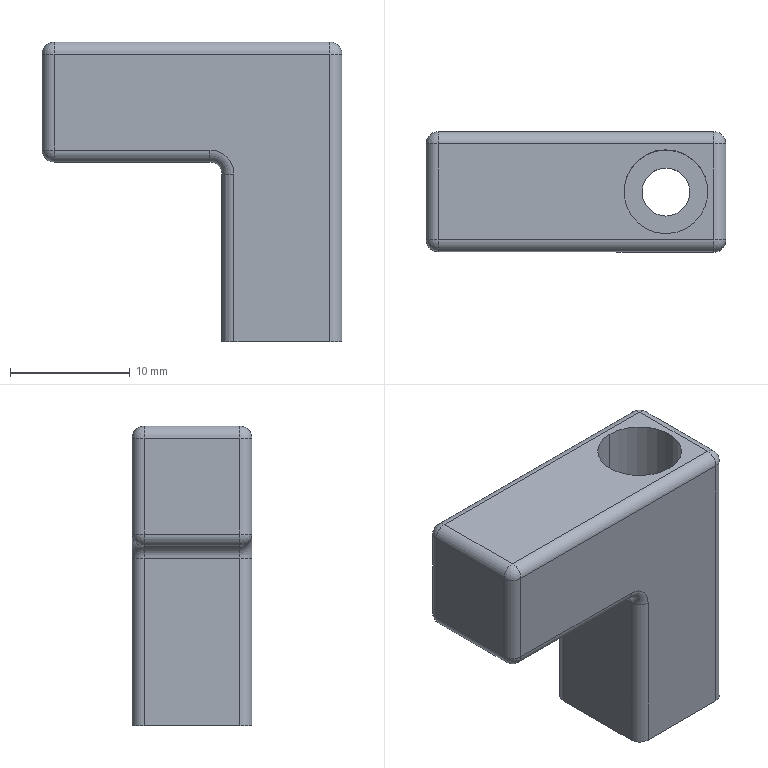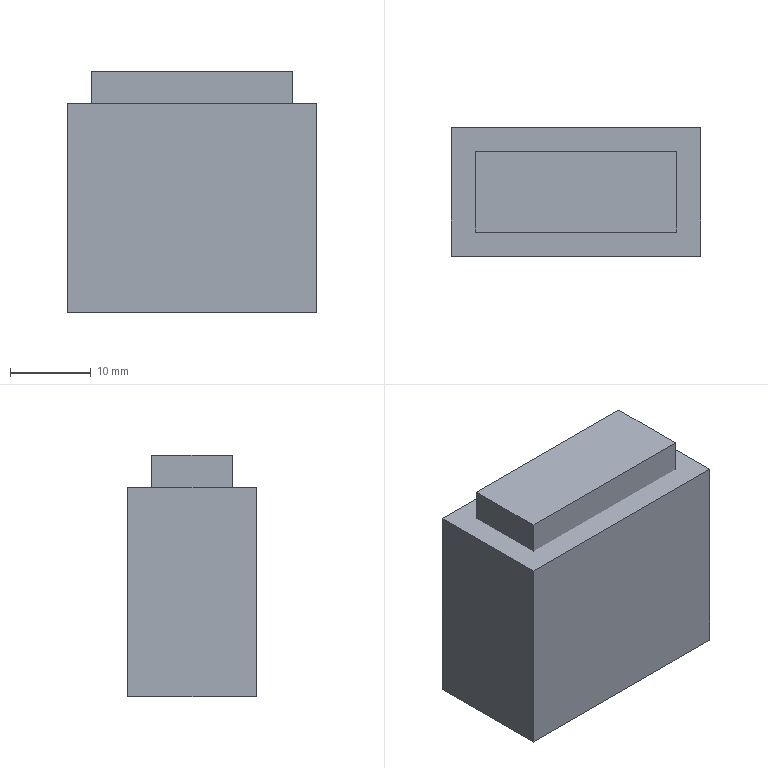CAM job | NX | 3-axis milling, drilling | part box 25 x 10 x 25 mm | stock box 31 x 16 x 30 mm
Tools:
number,name,description,diameter,corner_radius,flute_length,length,flutes
1,D63,Milling Tool-5 Parameters,63.0,0.0,50.0,75.0,2
9,D10,Milling Tool-5 Parameters,10.0,0.0,50.0,75.0,2
10,D10JING,Milling Tool-5 Parameters,10.0,0.0,50.0,75.0,2
8,D6R0.5,Milling Tool-5 Parameters,6.0,0.5,50.0,75.0,2
2,D4A45,Milling Tool-5 Parameters,4.0,0.0,2.0,2.0,2
14,4.0ZT,Drilling Tool,4.0,0.0,35.0,50.0,2
4,D4,Milling Tool-5 Parameters,4.0,0.0,50.0,75.0,2
Operations:
program,operation,operation_type,tool,method,geometry_group,spindle_rpm,surface_speed,feed_per_tooth,feed_cut,feed_plunge,cut_length_mm,path_length_mm,cut_time_min,machine_time_min
1,FLOOR_WALL,VolumeBased25DMillingOperation,D63,METHOD,A,6500.0,1286.0,0.0962,1250.0,100.0,106.0,126.0,0.0848,0.0868
1,ZLEVEL_PROFILE,ZLevelMilling,D10,METHOD,A,9500.0,298.0,0.1579,3000.0,1000.0,2614.871,2658.871,0.9035,0.9079
1,ZLEVEL_PROFILE_COPY_COPY,ZLevelMilling,D10JING,METHOD,A,9500.0,119.0,0.0632,1200.0,1000.0,324.188,487.93,0.2722,0.2886
1,ZLEVEL_PROFILE_COPY_1,ZLevelMilling,D6R0.5,METHOD,A,9500.0,179.0,0.1579,3000.0,1000.0,1946.433,1966.945,0.6509,0.653
1,DRILLING_COPY,Operation,D4A45,METHOD,A,5000.0,62.0,0.025,250.0,0.0,4.0,68.0,0.016,0.0224
1,DRILLING_COPY_COPY_COPY_COPY,Operation,4.0ZT,METHOD,A,1910.0,21.0,0.0471,180.0,0.0,30.702,121.403,0.1706,0.1796
1,HOLE_MILLING,CylinderMilling,D4,METHOD,A,9500.0,179.0,0.0658,1250.0,100.0,501.331,537.831,0.4011,0.4047
1,ZLEVEL_PROFILE_1_COPY_1_COPY,ZLevelMilling,D4A45,METHOD,A,9500.0,179.0,0.0526,1000.0,100.0,20.65,42.65,0.0207,0.0229
2,FLOOR_WALL_COPY,VolumeBased25DMillingOperation,D63,METHOD,B,6500.0,1286.0,0.0962,1250.0,100.0,500.0,1126.001,0.4,0.4626
2,FLOOR_WALL_1,VolumeBased25DMillingOperation,D10,METHOD,B,9500.0,298.0,0.1316,2500.0,1000.0,902.765,1140.262,0.4464,0.4701
2,FLOOR_WALL_2,VolumeBased25DMillingOperation,D10JING,METHOD,B,9500.0,119.0,0.0526,1000.0,100.0,97.121,293.388,0.0971,0.1167
2,ZLEVEL_PROFILE_COPY_COPY_COPY,ZLevelMilling,D10JING,METHOD,B,9500.0,119.0,0.0632,1200.0,1000.0,34.603,119.603,0.0295,0.038
2,ZLEVEL_PROFILE_COPY_1_COPY,ZLevelMilling,D6R0.5,METHOD,B,9500.0,179.0,0.1579,3000.0,1000.0,313.26,399.36,0.1066,0.1152
2,ZLEVEL_PROFILE_COPY_1_COPY_COPY,ZLevelMilling,D6R0.5,METHOD,B,9500.0,179.0,0.1579,3000.0,1000.0,1039.558,1128.07,0.3486,0.3574
2,ZLEVEL_PROFILE_1_COPY_1_COPY_COPY,ZLevelMilling,D4A45,METHOD,B,9500.0,179.0,0.0526,1000.0,100.0,59.159,187.062,0.0592,0.0719